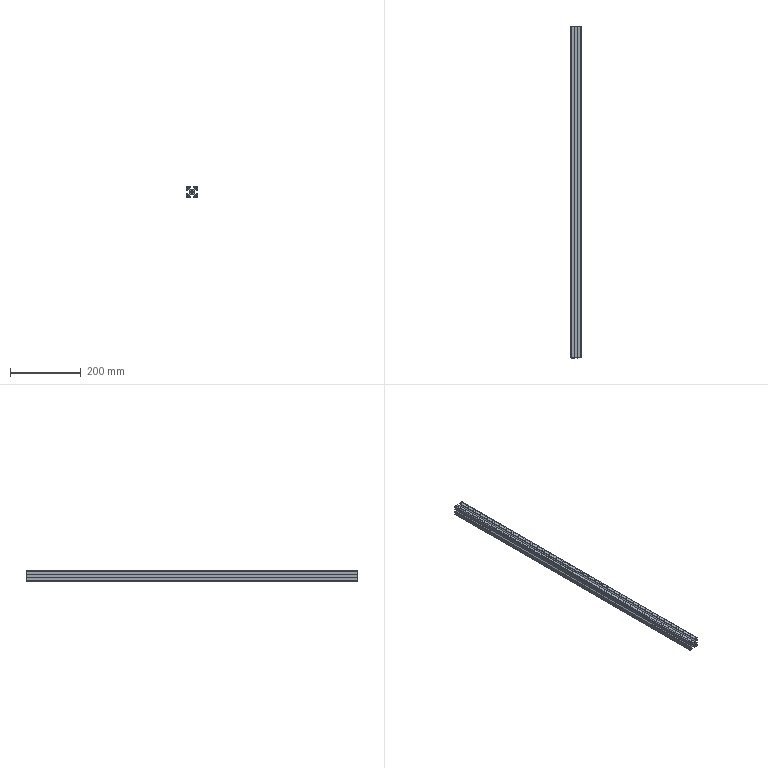Part | SolidWorks | features Extrusion 1 | 1 solid | 60 faces | box 30 x 940 x 30 mm | volume 312585 mm3 | plane 46 | cylinder 14 | commonest cylinder face diameters 4.2 x8 4 x4 6.8 x2